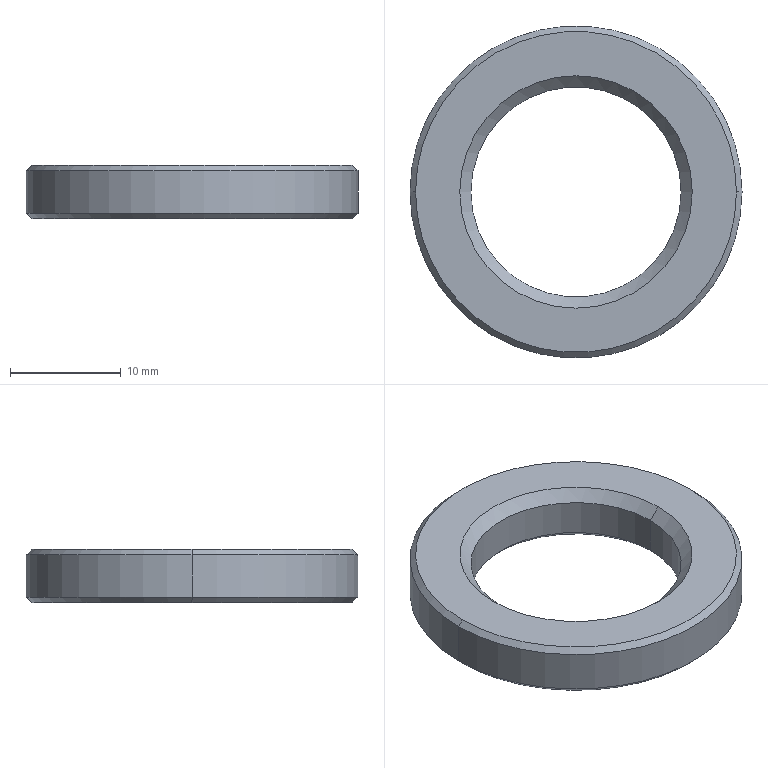Part | STEP file | 0230_Z_005_MRWZ12_2 | 1 solid | 26 faces | box 30 x 30 x 4.8 mm | volume 1915 mm3 | cylinder 12 | cone 8 | plane 6 | commonest cylinder face diameters 2.1 x8 19 x2 30 x2